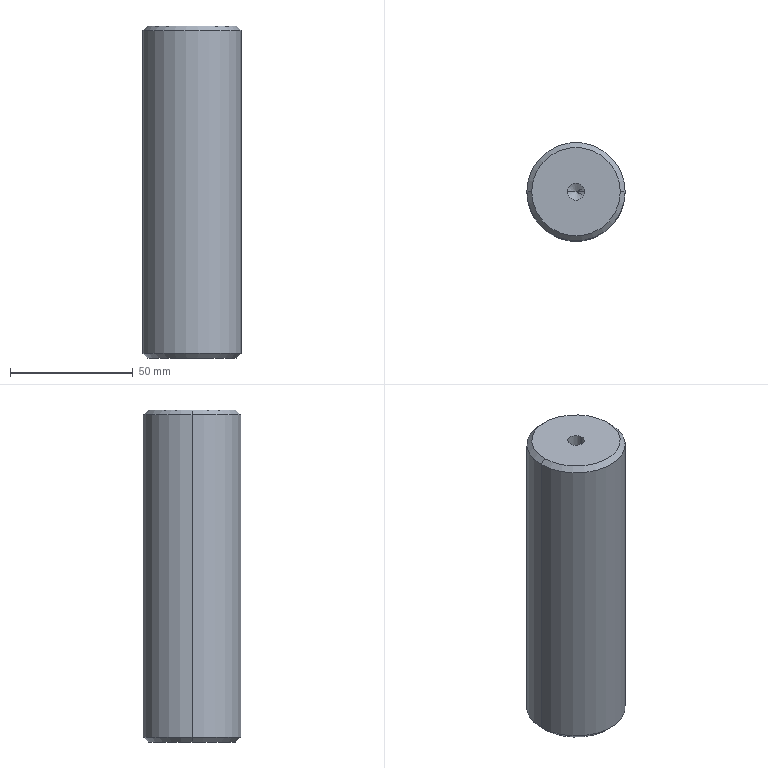Part | STEP file | 10-18 raised guide post | 1 solid | 16 faces | box 40 x 40 x 135 mm | volume 167676 mm3 | cone 8 | cylinder 6 | plane 2 | commonest cylinder face diameters 6.8 x4 40 x2
STEP:
#1=CARTESIAN_POINT('',(3.4,0.,-47.75));
#2=VERTEX_POINT('',#1);
#3=CARTESIAN_POINT('',(-3.4,0.,-47.75));
#4=VERTEX_POINT('',#3);
#5=CARTESIAN_POINT('',(0.,0.,-47.75));
#6=DIRECTION('',(0.,0.,-1.));
#7=DIRECTION('',(-1.,0.,0.));
#8=AXIS2_PLACEMENT_3D('',#5,#6,#7);
#9=CIRCLE('',#8,3.4);
#10=EDGE_CURVE('',#2,#4,#9,.T.);
#11=ORIENTED_EDGE('',*,*,#10,.F.);
#12=CARTESIAN_POINT('',(3.4,0.,-67.5));
#13=VERTEX_POINT('',#12);
#14=CARTESIAN_POINT('',(3.4,0.,-67.5));
#15=DIRECTION('',(0.,0.,-1.));
#16=VECTOR('',#15,1000.);
#17=LINE('',#14,#16);
#18=EDGE_CURVE('',#2,#13,#17,.T.);
#19=ORIENTED_EDGE('',*,*,#18,.T.);
#20=CARTESIAN_POINT('',(-3.4,0.,-67.5));
#21=VERTEX_POINT('',#20);
#22=CARTESIAN_POINT('',(0.,0.,-67.5));
#23=DIRECTION('',(0.,0.,-1.));
#24=DIRECTION('',(-1.,0.,0.));
#25=AXIS2_PLACEMENT_3D('',#22,#23,#24);
#26=CIRCLE('',#25,3.4);
#27=EDGE_CURVE('',#13,#21,#26,.T.);
#28=ORIENTED_EDGE('',*,*,#27,.T.);
#29=CARTESIAN_POINT('',(-3.4,0.,-67.5));
#30=DIRECTION('',(0.,0.,-1.));
#31=VECTOR('',#30,1000.);
#32=LINE('',#29,#31);
#33=EDGE_CURVE('',#4,#21,#32,.T.);
#34=ORIENTED_EDGE('',*,*,#33,.F.);
#35=EDGE_LOOP('',(#11,#19,#28,#34));
#36=FACE_OUTER_BOUND('',#35,.T.);
#37=CARTESIAN_POINT('',(0.,0.,-67.5));
#38=DIRECTION('',(0.,0.,-1.));
#39=DIRECTION('',(-1.,0.,0.));
#40=AXIS2_PLACEMENT_3D('',#37,#38,#39);
#41=CYLINDRICAL_SURFACE('',#40,3.4);
#42=ADVANCED_FACE('',(#36),#41,.F.);
#43=CARTESIAN_POINT('',(0.,0.,-45.707));
#44=VERTEX_POINT('',#43);
#45=CARTESIAN_POINT('',(-3.4,0.,-47.75));
#46=DIRECTION('',(-0.8572,0.,-0.515));
#47=VECTOR('',#46,1000.);
#48=LINE('',#45,#47);
#49=EDGE_CURVE('',#44,#4,#48,.T.);
#50=ORIENTED_EDGE('',*,*,#49,.F.);
#51=CARTESIAN_POINT('',(3.4,0.,-47.75));
#52=DIRECTION('',(0.8572,0.,-0.515));
#53=VECTOR('',#52,1000.);
#54=LINE('',#51,#53);
#55=EDGE_CURVE('',#44,#2,#54,.T.);
#56=ORIENTED_EDGE('',*,*,#55,.T.);
#57=ORIENTED_EDGE('',*,*,#10,.T.);
#58=EDGE_LOOP('',(#50,#56,#57));
#59=FACE_OUTER_BOUND('',#58,.T.);
#60=CARTESIAN_POINT('',(0.,0.,-47.75));
#61=DIRECTION('',(0.,0.,-1.));
#62=DIRECTION('',(-1.,0.,0.));
#63=AXIS2_PLACEMENT_3D('',#60,#61,#62);
#64=CONICAL_SURFACE('',#63,3.4,1.03);
#65=ADVANCED_FACE('',(#59),#64,.F.);
#66=CARTESIAN_POINT('',(-3.4,0.,47.75));
#67=VERTEX_POINT('',#66);
#68=CARTESIAN_POINT('',(3.4,0.,47.75));
#69=VERTEX_POINT('',#68);
#70=CARTESIAN_POINT('',(0.,0.,47.75));
#71=DIRECTION('',(0.,0.,1.));
#72=DIRECTION('',(1.,0.,0.));
#73=AXIS2_PLACEMENT_3D('',#70,#71,#72);
#74=CIRCLE('',#73,3.4);
#75=EDGE_CURVE('',#67,#69,#74,.T.);
#76=ORIENTED_EDGE('',*,*,#75,.F.);
#77=CARTESIAN_POINT('',(-3.4,0.,67.5));
#78=VERTEX_POINT('',#77);
#79=CARTESIAN_POINT('',(-3.4,0.,67.5));
#80=DIRECTION('',(0.,0.,1.));
#81=VECTOR('',#80,1000.);
#82=LINE('',#79,#81);
#83=EDGE_CURVE('',#67,#78,#82,.T.);
#84=ORIENTED_EDGE('',*,*,#83,.T.);
#85=CARTESIAN_POINT('',(3.4,0.,67.5));
#86=VERTEX_POINT('',#85);
#87=CARTESIAN_POINT('',(0.,0.,67.5));
#88=DIRECTION('',(0.,0.,1.));
#89=DIRECTION('',(1.,0.,0.));
#90=AXIS2_PLACEMENT_3D('',#87,#88,#89);
#91=CIRCLE('',#90,3.4);
#92=EDGE_CURVE('',#78,#86,#91,.T.);
#93=ORIENTED_EDGE('',*,*,#92,.T.);
#94=CARTESIAN_POINT('',(3.4,0.,67.5));
#95=DIRECTION('',(0.,0.,1.));
#96=VECTOR('',#95,1000.);
#97=LINE('',#94,#96);
#98=EDGE_CURVE('',#69,#86,#97,.T.);
#99=ORIENTED_EDGE('',*,*,#98,.F.);
#100=EDGE_LOOP('',(#76,#84,#93,#99));
#101=FACE_OUTER_BOUND('',#100,.T.);
#102=CARTESIAN_POINT('',(0.,0.,67.5));
#103=DIRECTION('',(0.,0.,1.));
#104=DIRECTION('',(1.,0.,0.));
#105=AXIS2_PLACEMENT_3D('',#102,#103,#104);
#106=CYLINDRICAL_SURFACE('',#105,3.4);
#107=ADVANCED_FACE('',(#101),#106,.F.);
#108=CARTESIAN_POINT('',(0.,0.,45.707));
#109=VERTEX_POINT('',#108);
#110=CARTESIAN_POINT('',(3.4,0.,47.75));
#111=DIRECTION('',(0.8572,0.,0.515));
#112=VECTOR('',#111,1000.);
#113=LINE('',#110,#112);
#114=EDGE_CURVE('',#109,#69,#113,.T.);
#115=ORIENTED_EDGE('',*,*,#114,.F.);
#116=CARTESIAN_POINT('',(-3.4,0.,47.75));
#117=DIRECTION('',(-0.8572,0.,0.515));
#118=VECTOR('',#117,1000.);
#119=LINE('',#116,#118);
#120=EDGE_CURVE('',#109,#67,#119,.T.);
#121=ORIENTED_EDGE('',*,*,#120,.T.);
#122=ORIENTED_EDGE('',*,*,#75,.T.);
#123=EDGE_LOOP('',(#115,#121,#122));
#124=FACE_OUTER_BOUND('',#123,.T.);
#125=CARTESIAN_POINT('',(0.,0.,47.75));
#126=DIRECTION('',(0.,0.,1.));
#127=DIRECTION('',(1.,0.,0.));
#128=AXIS2_PLACEMENT_3D('',#125,#126,#127);
#129=CONICAL_SURFACE('',#128,3.4,1.03);
#130=ADVANCED_FACE('',(#124),#129,.F.);
#131=CARTESIAN_POINT('',(-18.,0.,-67.5));
#132=VERTEX_POINT('',#131);
#133=CARTESIAN_POINT('',(18.,0.,-67.5));
#134=VERTEX_POINT('',#133);
#135=CARTESIAN_POINT('',(0.,0.,-67.5));
#136=DIRECTION('',(0.,0.,-1.));
#137=DIRECTION('',(1.,0.,0.));
#138=AXIS2_PLACEMENT_3D('',#135,#136,#137);
#139=CIRCLE('',#138,18.);
#140=EDGE_CURVE('',#132,#134,#139,.T.);
#141=ORIENTED_EDGE('',*,*,#140,.F.);
#142=CARTESIAN_POINT('',(-20.,0.,-65.5));
#143=VERTEX_POINT('',#142);
#144=CARTESIAN_POINT('',(-20.,0.,-65.5));
#145=DIRECTION('',(-0.7071,0.,0.7071));
#146=VECTOR('',#145,1000.);
#147=LINE('',#144,#146);
#148=EDGE_CURVE('',#132,#143,#147,.T.);
#149=ORIENTED_EDGE('',*,*,#148,.T.);
#150=CARTESIAN_POINT('',(20.,0.,-65.5));
#151=VERTEX_POINT('',#150);
#152=CARTESIAN_POINT('',(0.,0.,-65.5));
#153=DIRECTION('',(0.,0.,1.));
#154=DIRECTION('',(1.,0.,0.));
#155=AXIS2_PLACEMENT_3D('',#152,#153,#154);
#156=CIRCLE('',#155,20.);
#157=EDGE_CURVE('',#151,#143,#156,.T.);
#158=ORIENTED_EDGE('',*,*,#157,.F.);
#159=CARTESIAN_POINT('',(20.,0.,-65.5));
#160=DIRECTION('',(0.7071,0.,0.7071));
#161=VECTOR('',#160,1000.);
#162=LINE('',#159,#161);
#163=EDGE_CURVE('',#134,#151,#162,.T.);
#164=ORIENTED_EDGE('',*,*,#163,.F.);
#165=EDGE_LOOP('',(#141,#149,#158,#164));
#166=FACE_OUTER_BOUND('',#165,.T.);
#167=CARTESIAN_POINT('',(0.,0.,-65.5));
#168=DIRECTION('',(0.,0.,1.));
#169=DIRECTION('',(1.,0.,0.));
#170=AXIS2_PLACEMENT_3D('',#167,#168,#169);
#171=CONICAL_SURFACE('',#170,20.,0.7854);
#172=ADVANCED_FACE('',(#166),#171,.T.);
#173=CARTESIAN_POINT('',(18.,0.,67.5));
#174=VERTEX_POINT('',#173);
#175=CARTESIAN_POINT('',(-18.,0.,67.5));
#176=VERTEX_POINT('',#175);
#177=CARTESIAN_POINT('',(0.,0.,67.5));
#178=DIRECTION('',(0.,0.,1.));
#179=DIRECTION('',(1.,0.,0.));
#180=AXIS2_PLACEMENT_3D('',#177,#178,#179);
#181=CIRCLE('',#180,18.);
#182=EDGE_CURVE('',#174,#176,#181,.T.);
#183=ORIENTED_EDGE('',*,*,#182,.F.);
#184=CARTESIAN_POINT('',(20.,0.,65.5));
#185=VERTEX_POINT('',#184);
#186=CARTESIAN_POINT('',(18.,0.,67.5));
#187=DIRECTION('',(0.7071,0.,-0.7071));
#188=VECTOR('',#187,1000.);
#189=LINE('',#186,#188);
#190=EDGE_CURVE('',#174,#185,#189,.T.);
#191=ORIENTED_EDGE('',*,*,#190,.T.);
#192=CARTESIAN_POINT('',(-20.,0.,65.5));
#193=VERTEX_POINT('',#192);
#194=CARTESIAN_POINT('',(0.,0.,65.5));
#195=DIRECTION('',(0.,0.,-1.));
#196=DIRECTION('',(1.,0.,0.));
#197=AXIS2_PLACEMENT_3D('',#194,#195,#196);
#198=CIRCLE('',#197,20.);
#199=EDGE_CURVE('',#193,#185,#198,.T.);
#200=ORIENTED_EDGE('',*,*,#199,.F.);
#201=CARTESIAN_POINT('',(-18.,0.,67.5));
#202=DIRECTION('',(-0.7071,0.,-0.7071));
#203=VECTOR('',#202,1000.);
#204=LINE('',#201,#203);
#205=EDGE_CURVE('',#176,#193,#204,.T.);
#206=ORIENTED_EDGE('',*,*,#205,.F.);
#207=EDGE_LOOP('',(#183,#191,#200,#206));
#208=FACE_OUTER_BOUND('',#207,.T.);
#209=CARTESIAN_POINT('',(0.,0.,67.5));
#210=DIRECTION('',(0.,0.,-1.));
#211=DIRECTION('',(-1.,0.,0.));
#212=AXIS2_PLACEMENT_3D('',#209,#210,#211);
#213=CONICAL_SURFACE('',#212,18.,0.7854);
#214=ADVANCED_FACE('',(#208),#213,.T.);
#215=ORIENTED_EDGE('',*,*,#199,.T.);
#216=CARTESIAN_POINT('',(20.,0.,67.5));
#217=DIRECTION('',(0.,0.,-1.));
#218=VECTOR('',#217,1000.);
#219=LINE('',#216,#218);
#220=EDGE_CURVE('',#185,#151,#219,.T.);
#221=ORIENTED_EDGE('',*,*,#220,.T.);
#222=ORIENTED_EDGE('',*,*,#157,.T.);
#223=CARTESIAN_POINT('',(-20.,0.,67.5));
#224=DIRECTION('',(0.,0.,-1.));
#225=VECTOR('',#224,1000.);
#226=LINE('',#223,#225);
#227=EDGE_CURVE('',#193,#143,#226,.T.);
#228=ORIENTED_EDGE('',*,*,#227,.F.);
#229=EDGE_LOOP('',(#215,#221,#222,#228));
#230=FACE_OUTER_BOUND('',#229,.T.);
#231=CARTESIAN_POINT('',(0.,0.,67.5));
#232=DIRECTION('',(0.,0.,-1.));
#233=DIRECTION('',(-1.,0.,0.));
#234=AXIS2_PLACEMENT_3D('',#231,#232,#233);
#235=CYLINDRICAL_SURFACE('',#234,20.);
#236=ADVANCED_FACE('',(#230),#235,.T.);
#237=ORIENTED_EDGE('',*,*,#220,.F.);
#238=CARTESIAN_POINT('',(0.,0.,65.5));
#239=DIRECTION('',(0.,0.,-1.));
#240=DIRECTION('',(1.,0.,0.));
#241=AXIS2_PLACEMENT_3D('',#238,#239,#240);
#242=CIRCLE('',#241,20.);
#243=EDGE_CURVE('',#185,#193,#242,.T.);
#244=ORIENTED_EDGE('',*,*,#243,.T.);
#245=ORIENTED_EDGE('',*,*,#227,.T.);
#246=CARTESIAN_POINT('',(0.,0.,-65.5));
#247=DIRECTION('',(0.,0.,1.));
#248=DIRECTION('',(1.,0.,0.));
#249=AXIS2_PLACEMENT_3D('',#246,#247,#248);
#250=CIRCLE('',#249,20.);
#251=EDGE_CURVE('',#143,#151,#250,.T.);
#252=ORIENTED_EDGE('',*,*,#251,.T.);
#253=EDGE_LOOP('',(#237,#244,#245,#252));
#254=FACE_OUTER_BOUND('',#253,.T.);
#255=CARTESIAN_POINT('',(0.,0.,67.5));
#256=DIRECTION('',(0.,0.,-1.));
#257=DIRECTION('',(-1.,0.,0.));
#258=AXIS2_PLACEMENT_3D('',#255,#256,#257);
#259=CYLINDRICAL_SURFACE('',#258,20.);
#260=ADVANCED_FACE('',(#254),#259,.T.);
#261=CARTESIAN_POINT('',(0.,0.,67.5));
#262=DIRECTION('',(0.,0.,1.));
#263=DIRECTION('',(1.,0.,0.));
#264=AXIS2_PLACEMENT_3D('',#261,#262,#263);
#265=CIRCLE('',#264,3.4);
#266=EDGE_CURVE('',#86,#78,#265,.T.);
#267=ORIENTED_EDGE('',*,*,#266,.F.);
#268=ORIENTED_EDGE('',*,*,#92,.F.);
#269=EDGE_LOOP('',(#267,#268));
#270=FACE_BOUND('',#269,.T.);
#271=CARTESIAN_POINT('',(0.,0.,67.5));
#272=DIRECTION('',(0.,0.,1.));
#273=DIRECTION('',(1.,0.,0.));
#274=AXIS2_PLACEMENT_3D('',#271,#272,#273);
#275=CIRCLE('',#274,18.);
#276=EDGE_CURVE('',#176,#174,#275,.T.);
#277=ORIENTED_EDGE('',*,*,#276,.T.);
#278=ORIENTED_EDGE('',*,*,#182,.T.);
#279=EDGE_LOOP('',(#277,#278));
#280=FACE_OUTER_BOUND('',#279,.T.);
#281=CARTESIAN_POINT('',(0.,0.,67.5));
#282=DIRECTION('',(0.,0.,1.));
#283=DIRECTION('',(1.,0.,0.));
#284=AXIS2_PLACEMENT_3D('',#281,#282,#283);
#285=PLANE('',#284);
#286=ADVANCED_FACE('',(#270,#280),#285,.T.);
#287=CARTESIAN_POINT('',(0.,0.,-67.5));
#288=DIRECTION('',(0.,0.,-1.));
#289=DIRECTION('',(-1.,0.,0.));
#290=AXIS2_PLACEMENT_3D('',#287,#288,#289);
#291=CIRCLE('',#290,3.4);
#292=EDGE_CURVE('',#21,#13,#291,.T.);
#293=ORIENTED_EDGE('',*,*,#292,.F.);
#294=ORIENTED_EDGE('',*,*,#27,.F.);
#295=EDGE_LOOP('',(#293,#294));
#296=FACE_BOUND('',#295,.T.);
#297=CARTESIAN_POINT('',(0.,0.,-67.5));
#298=DIRECTION('',(0.,0.,-1.));
#299=DIRECTION('',(1.,0.,0.));
#300=AXIS2_PLACEMENT_3D('',#297,#298,#299);
#301=CIRCLE('',#300,18.);
#302=EDGE_CURVE('',#134,#132,#301,.T.);
#303=ORIENTED_EDGE('',*,*,#302,.T.);
#304=ORIENTED_EDGE('',*,*,#140,.T.);
#305=EDGE_LOOP('',(#303,#304));
#306=FACE_OUTER_BOUND('',#305,.T.);
#307=CARTESIAN_POINT('',(0.,0.,-67.5));
#308=DIRECTION('',(0.,0.,1.));
#309=DIRECTION('',(1.,0.,0.));
#310=AXIS2_PLACEMENT_3D('',#307,#308,#309);
#311=PLANE('',#310);
#312=ADVANCED_FACE('',(#296,#306),#311,.F.);
#313=ORIENTED_EDGE('',*,*,#190,.F.);
#314=ORIENTED_EDGE('',*,*,#276,.F.);
#315=ORIENTED_EDGE('',*,*,#205,.T.);
#316=ORIENTED_EDGE('',*,*,#243,.F.);
#317=EDGE_LOOP('',(#313,#314,#315,#316));
#318=FACE_OUTER_BOUND('',#317,.T.);
#319=CARTESIAN_POINT('',(0.,0.,67.5));
#320=DIRECTION('',(0.,0.,-1.));
#321=DIRECTION('',(-1.,0.,0.));
#322=AXIS2_PLACEMENT_3D('',#319,#320,#321);
#323=CONICAL_SURFACE('',#322,18.,0.7854);
#324=ADVANCED_FACE('',(#318),#323,.T.);
#325=ORIENTED_EDGE('',*,*,#148,.F.);
#326=ORIENTED_EDGE('',*,*,#302,.F.);
#327=ORIENTED_EDGE('',*,*,#163,.T.);
#328=ORIENTED_EDGE('',*,*,#251,.F.);
#329=EDGE_LOOP('',(#325,#326,#327,#328));
#330=FACE_OUTER_BOUND('',#329,.T.);
#331=CARTESIAN_POINT('',(0.,0.,-65.5));
#332=DIRECTION('',(0.,0.,1.));
#333=DIRECTION('',(1.,0.,0.));
#334=AXIS2_PLACEMENT_3D('',#331,#332,#333);
#335=CONICAL_SURFACE('',#334,20.,0.7854);
#336=ADVANCED_FACE('',(#330),#335,.T.);
#337=ORIENTED_EDGE('',*,*,#120,.F.);
#338=ORIENTED_EDGE('',*,*,#114,.T.);
#339=CARTESIAN_POINT('',(0.,0.,47.75));
#340=DIRECTION('',(0.,0.,1.));
#341=DIRECTION('',(1.,0.,0.));
#342=AXIS2_PLACEMENT_3D('',#339,#340,#341);
#343=CIRCLE('',#342,3.4);
#344=EDGE_CURVE('',#69,#67,#343,.T.);
#345=ORIENTED_EDGE('',*,*,#344,.T.);
#346=EDGE_LOOP('',(#337,#338,#345));
#347=FACE_OUTER_BOUND('',#346,.T.);
#348=CARTESIAN_POINT('',(0.,0.,47.75));
#349=DIRECTION('',(0.,0.,1.));
#350=DIRECTION('',(1.,0.,0.));
#351=AXIS2_PLACEMENT_3D('',#348,#349,#350);
#352=CONICAL_SURFACE('',#351,3.4,1.03);
#353=ADVANCED_FACE('',(#347),#352,.F.);
#354=ORIENTED_EDGE('',*,*,#83,.F.);
#355=ORIENTED_EDGE('',*,*,#344,.F.);
#356=ORIENTED_EDGE('',*,*,#98,.T.);
#357=ORIENTED_EDGE('',*,*,#266,.T.);
#358=EDGE_LOOP('',(#354,#355,#356,#357));
#359=FACE_OUTER_BOUND('',#358,.T.);
#360=CARTESIAN_POINT('',(0.,0.,67.5));
#361=DIRECTION('',(0.,0.,1.));
#362=DIRECTION('',(1.,0.,0.));
#363=AXIS2_PLACEMENT_3D('',#360,#361,#362);
#364=CYLINDRICAL_SURFACE('',#363,3.4);
#365=ADVANCED_FACE('',(#359),#364,.F.);
#366=ORIENTED_EDGE('',*,*,#55,.F.);
#367=ORIENTED_EDGE('',*,*,#49,.T.);
#368=CARTESIAN_POINT('',(0.,0.,-47.75));
#369=DIRECTION('',(0.,0.,-1.));
#370=DIRECTION('',(-1.,0.,0.));
#371=AXIS2_PLACEMENT_3D('',#368,#369,#370);
#372=CIRCLE('',#371,3.4);
#373=EDGE_CURVE('',#4,#2,#372,.T.);
#374=ORIENTED_EDGE('',*,*,#373,.T.);
#375=EDGE_LOOP('',(#366,#367,#374));
#376=FACE_OUTER_BOUND('',#375,.T.);
#377=CARTESIAN_POINT('',(0.,0.,-47.75));
#378=DIRECTION('',(0.,0.,-1.));
#379=DIRECTION('',(-1.,0.,0.));
#380=AXIS2_PLACEMENT_3D('',#377,#378,#379);
#381=CONICAL_SURFACE('',#380,3.4,1.03);
#382=ADVANCED_FACE('',(#376),#381,.F.);
#383=ORIENTED_EDGE('',*,*,#18,.F.);
#384=ORIENTED_EDGE('',*,*,#373,.F.);
#385=ORIENTED_EDGE('',*,*,#33,.T.);
#386=ORIENTED_EDGE('',*,*,#292,.T.);
#387=EDGE_LOOP('',(#383,#384,#385,#386));
#388=FACE_OUTER_BOUND('',#387,.T.);
#389=CARTESIAN_POINT('',(0.,0.,-67.5));
#390=DIRECTION('',(0.,0.,-1.));
#391=DIRECTION('',(-1.,0.,0.));
#392=AXIS2_PLACEMENT_3D('',#389,#390,#391);
#393=CYLINDRICAL_SURFACE('',#392,3.4);
#394=ADVANCED_FACE('',(#388),#393,.F.);
#395=CLOSED_SHELL('',(#42,#65,#107,#130,#172,#214,#236,#260,#286,#312,#324,#336,#353,#365,#382,#394));
#396=MANIFOLD_SOLID_BREP('',#395);
#397=CARTESIAN_POINT('',(0.,0.,0.));
#398=DIRECTION('',(0.,0.,1.));
#399=DIRECTION('',(1.,0.,0.));
#400=AXIS2_PLACEMENT_3D('',#397,#398,#399);
#401=(LENGTH_UNIT()NAMED_UNIT(*)SI_UNIT(.MILLI.,.METRE.));
#402=UNCERTAINTY_MEASURE_WITH_UNIT(LENGTH_MEASURE(0.00001),#401,'','');
#403=(NAMED_UNIT(*)PLANE_ANGLE_UNIT()SI_UNIT($,.RADIAN.));
#404=(NAMED_UNIT(*)SI_UNIT($,.STERADIAN.)SOLID_ANGLE_UNIT());
#405=(GEOMETRIC_REPRESENTATION_CONTEXT(3)GLOBAL_UNCERTAINTY_ASSIGNED_CONTEXT((#402))GLOBAL_UNIT_ASSIGNED_CONTEXT((#401,#403,#404))REPRESENTATION_CONTEXT('',''));
#406=ADVANCED_BREP_SHAPE_REPRESENTATION('',(#396,#400),#405);